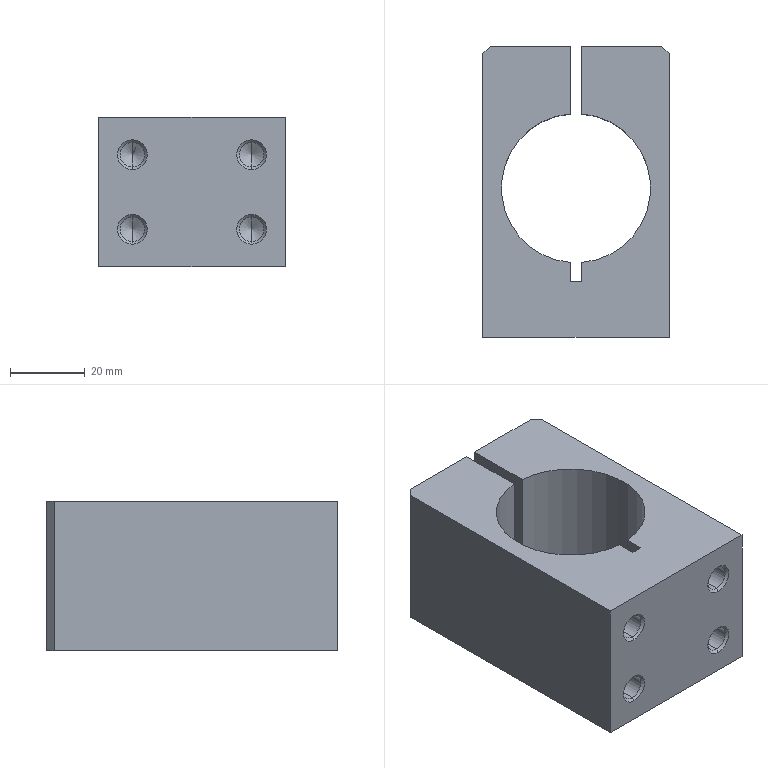Part | STEP file | fBY02F02M-00-03A | 1 solid | 62 faces | box 50 x 78 x 40 mm | volume 94734 mm3 | cone 24 | cylinder 22 | plane 16 | commonest cylinder face diameters 6.647 x12 9 x4 14 x4 40 x2